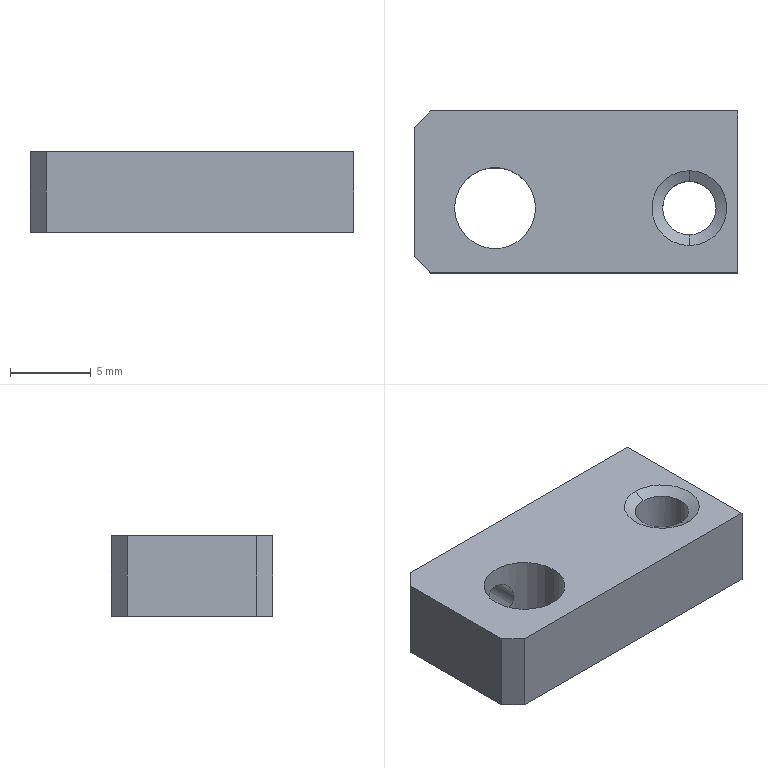Part | NX | 1 solid | 18 faces | box 20 x 10 x 5 mm | volume 834.465 mm3 | plane 8 | cylinder 6 | cone 4 | commonest cylinder face diameters 2.5 x2 3.3 x2 5 x2
STEP:
#1=CARTESIAN_POINT('',(-5.,-3.,0.));
#2=VERTEX_POINT('',#1);
#3=CARTESIAN_POINT('',(-5.,5.,0.));
#4=VERTEX_POINT('',#3);
#5=CARTESIAN_POINT('',(-5.,0.,0.));
#6=DIRECTION('',(0.,1.,0.));
#7=VECTOR('',#6,1000.);
#8=LINE('',#5,#7);
#9=EDGE_CURVE('',#2,#4,#8,.T.);
#10=ORIENTED_EDGE('',*,*,#9,.T.);
#11=CARTESIAN_POINT('',(-4.,6.,0.));
#12=VERTEX_POINT('',#11);
#13=CARTESIAN_POINT('',(-10.,0.,0.));
#14=DIRECTION('',(0.7071,0.7071,0.));
#15=VECTOR('',#14,1000.);
#16=LINE('',#13,#15);
#17=EDGE_CURVE('',#4,#12,#16,.T.);
#18=ORIENTED_EDGE('',*,*,#17,.T.);
#19=CARTESIAN_POINT('',(15.,6.,0.));
#20=VERTEX_POINT('',#19);
#21=CARTESIAN_POINT('',(0.,6.,0.));
#22=DIRECTION('',(-1.,0.,0.));
#23=VECTOR('',#22,1000.);
#24=LINE('',#21,#23);
#25=EDGE_CURVE('',#20,#12,#24,.T.);
#26=ORIENTED_EDGE('',*,*,#25,.F.);
#27=CARTESIAN_POINT('',(15.,-4.,0.));
#28=VERTEX_POINT('',#27);
#29=CARTESIAN_POINT('',(15.,0.,0.));
#30=DIRECTION('',(0.,-1.,0.));
#31=VECTOR('',#30,1000.);
#32=LINE('',#29,#31);
#33=EDGE_CURVE('',#20,#28,#32,.T.);
#34=ORIENTED_EDGE('',*,*,#33,.T.);
#35=CARTESIAN_POINT('',(-4.,-4.,0.));
#36=VERTEX_POINT('',#35);
#37=CARTESIAN_POINT('',(0.,-4.,0.));
#38=DIRECTION('',(-1.,0.,0.));
#39=VECTOR('',#38,1000.);
#40=LINE('',#37,#39);
#41=EDGE_CURVE('',#28,#36,#40,.T.);
#42=ORIENTED_EDGE('',*,*,#41,.T.);
#43=CARTESIAN_POINT('',(-8.,0.,0.));
#44=DIRECTION('',(-0.7071,0.7071,0.));
#45=VECTOR('',#44,1000.);
#46=LINE('',#43,#45);
#47=EDGE_CURVE('',#36,#2,#46,.T.);
#48=ORIENTED_EDGE('',*,*,#47,.T.);
#49=EDGE_LOOP('',(#10,#18,#26,#34,#42,#48));
#50=FACE_BOUND('',#49,.T.);
#51=CARTESIAN_POINT('',(-2.5,0.,0.));
#52=VERTEX_POINT('',#51);
#53=CARTESIAN_POINT('',(2.5,0.,0.));
#54=VERTEX_POINT('',#53);
#55=CARTESIAN_POINT('',(0.,0.,0.));
#56=DIRECTION('',(0.,0.,1.));
#57=DIRECTION('',(1.,0.,0.));
#58=AXIS2_PLACEMENT_3D('',#55,#56,#57);
#59=CIRCLE('',#58,2.5);
#60=EDGE_CURVE('',#52,#54,#59,.T.);
#61=ORIENTED_EDGE('',*,*,#60,.T.);
#62=CARTESIAN_POINT('',(0.,0.,0.));
#63=DIRECTION('',(0.,0.,1.));
#64=DIRECTION('',(1.,0.,0.));
#65=AXIS2_PLACEMENT_3D('',#62,#63,#64);
#66=CIRCLE('',#65,2.5);
#67=EDGE_CURVE('',#54,#52,#66,.T.);
#68=ORIENTED_EDGE('',*,*,#67,.T.);
#69=EDGE_LOOP('',(#61,#68));
#70=FACE_BOUND('',#69,.T.);
#71=CARTESIAN_POINT('',(10.35,0.,0.));
#72=VERTEX_POINT('',#71);
#73=CARTESIAN_POINT('',(13.65,0.,0.));
#74=VERTEX_POINT('',#73);
#75=CARTESIAN_POINT('',(12.,0.,0.));
#76=DIRECTION('',(0.,0.,1.));
#77=DIRECTION('',(-1.,0.,0.));
#78=AXIS2_PLACEMENT_3D('',#75,#76,#77);
#79=CIRCLE('',#78,1.65);
#80=EDGE_CURVE('',#72,#74,#79,.T.);
#81=ORIENTED_EDGE('',*,*,#80,.T.);
#82=CARTESIAN_POINT('',(12.,0.,0.));
#83=DIRECTION('',(0.,0.,1.));
#84=DIRECTION('',(-1.,0.,0.));
#85=AXIS2_PLACEMENT_3D('',#82,#83,#84);
#86=CIRCLE('',#85,1.65);
#87=EDGE_CURVE('',#74,#72,#86,.T.);
#88=ORIENTED_EDGE('',*,*,#87,.T.);
#89=EDGE_LOOP('',(#81,#88));
#90=FACE_BOUND('',#89,.T.);
#91=CARTESIAN_POINT('',(0.,0.,0.));
#92=DIRECTION('',(0.,0.,1.));
#93=DIRECTION('',(1.,0.,0.));
#94=AXIS2_PLACEMENT_3D('',#91,#92,#93);
#95=PLANE('',#94);
#96=ADVANCED_FACE('',(#50,#70,#90),#95,.F.);
#97=ORIENTED_EDGE('',*,*,#9,.F.);
#98=CARTESIAN_POINT('',(-5.,-3.,5.));
#99=VERTEX_POINT('',#98);
#100=CARTESIAN_POINT('',(-5.,-3.,5.));
#101=DIRECTION('',(0.,0.,-1.));
#102=VECTOR('',#101,1000.);
#103=LINE('',#100,#102);
#104=EDGE_CURVE('',#99,#2,#103,.T.);
#105=ORIENTED_EDGE('',*,*,#104,.F.);
#106=CARTESIAN_POINT('',(-5.,5.,5.));
#107=VERTEX_POINT('',#106);
#108=CARTESIAN_POINT('',(-5.,0.,5.));
#109=DIRECTION('',(0.,1.,0.));
#110=VECTOR('',#109,1000.);
#111=LINE('',#108,#110);
#112=EDGE_CURVE('',#99,#107,#111,.T.);
#113=ORIENTED_EDGE('',*,*,#112,.T.);
#114=CARTESIAN_POINT('',(-5.,5.,5.));
#115=DIRECTION('',(0.,0.,-1.));
#116=VECTOR('',#115,1000.);
#117=LINE('',#114,#116);
#118=EDGE_CURVE('',#107,#4,#117,.T.);
#119=ORIENTED_EDGE('',*,*,#118,.T.);
#120=EDGE_LOOP('',(#97,#105,#113,#119));
#121=FACE_BOUND('',#120,.T.);
#122=CARTESIAN_POINT('',(-5.,6.,0.));
#123=DIRECTION('',(-1.,0.,0.));
#124=DIRECTION('',(0.,0.,1.));
#125=AXIS2_PLACEMENT_3D('',#122,#123,#124);
#126=PLANE('',#125);
#127=ADVANCED_FACE('',(#121),#126,.T.);
#128=ORIENTED_EDGE('',*,*,#118,.F.);
#129=CARTESIAN_POINT('',(-4.,6.,5.));
#130=VERTEX_POINT('',#129);
#131=CARTESIAN_POINT('',(-10.,0.,5.));
#132=DIRECTION('',(0.7071,0.7071,0.));
#133=VECTOR('',#132,1000.);
#134=LINE('',#131,#133);
#135=EDGE_CURVE('',#107,#130,#134,.T.);
#136=ORIENTED_EDGE('',*,*,#135,.T.);
#137=CARTESIAN_POINT('',(-4.,6.,0.));
#138=DIRECTION('',(0.,0.,-1.));
#139=VECTOR('',#138,1000.);
#140=LINE('',#137,#139);
#141=EDGE_CURVE('',#130,#12,#140,.T.);
#142=ORIENTED_EDGE('',*,*,#141,.T.);
#143=ORIENTED_EDGE('',*,*,#17,.F.);
#144=EDGE_LOOP('',(#128,#136,#142,#143));
#145=FACE_BOUND('',#144,.T.);
#146=CARTESIAN_POINT('',(-5.,5.,0.));
#147=DIRECTION('',(-0.7071,0.7071,0.));
#148=DIRECTION('',(0.,0.,1.));
#149=AXIS2_PLACEMENT_3D('',#146,#147,#148);
#150=PLANE('',#149);
#151=ADVANCED_FACE('',(#145),#150,.T.);
#152=ORIENTED_EDGE('',*,*,#25,.T.);
#153=ORIENTED_EDGE('',*,*,#141,.F.);
#154=CARTESIAN_POINT('',(15.,6.,5.));
#155=VERTEX_POINT('',#154);
#156=CARTESIAN_POINT('',(0.,6.,5.));
#157=DIRECTION('',(-1.,0.,0.));
#158=VECTOR('',#157,1000.);
#159=LINE('',#156,#158);
#160=EDGE_CURVE('',#155,#130,#159,.T.);
#161=ORIENTED_EDGE('',*,*,#160,.F.);
#162=CARTESIAN_POINT('',(15.,6.,0.));
#163=DIRECTION('',(0.,0.,1.));
#164=VECTOR('',#163,1000.);
#165=LINE('',#162,#164);
#166=EDGE_CURVE('',#20,#155,#165,.T.);
#167=ORIENTED_EDGE('',*,*,#166,.F.);
#168=EDGE_LOOP('',(#152,#153,#161,#167));
#169=FACE_BOUND('',#168,.T.);
#170=CARTESIAN_POINT('',(-1.7,6.,2.5));
#171=VERTEX_POINT('',#170);
#172=CARTESIAN_POINT('',(1.7,6.,2.5));
#173=VERTEX_POINT('',#172);
#174=CARTESIAN_POINT('',(0.,6.,2.5));
#175=DIRECTION('',(0.,1.,0.));
#176=DIRECTION('',(1.,0.,0.));
#177=AXIS2_PLACEMENT_3D('',#174,#175,#176);
#178=CIRCLE('',#177,1.7);
#179=EDGE_CURVE('',#171,#173,#178,.T.);
#180=ORIENTED_EDGE('',*,*,#179,.F.);
#181=CARTESIAN_POINT('',(0.,6.,2.5));
#182=DIRECTION('',(0.,1.,0.));
#183=DIRECTION('',(1.,0.,0.));
#184=AXIS2_PLACEMENT_3D('',#181,#182,#183);
#185=CIRCLE('',#184,1.7);
#186=EDGE_CURVE('',#173,#171,#185,.T.);
#187=ORIENTED_EDGE('',*,*,#186,.F.);
#188=EDGE_LOOP('',(#180,#187));
#189=FACE_BOUND('',#188,.T.);
#190=CARTESIAN_POINT('',(15.,6.,0.));
#191=DIRECTION('',(0.,1.,0.));
#192=DIRECTION('',(1.,0.,0.));
#193=AXIS2_PLACEMENT_3D('',#190,#191,#192);
#194=PLANE('',#193);
#195=ADVANCED_FACE('',(#169,#189),#194,.T.);
#196=ORIENTED_EDGE('',*,*,#33,.F.);
#197=ORIENTED_EDGE('',*,*,#166,.T.);
#198=CARTESIAN_POINT('',(15.,-4.,5.));
#199=VERTEX_POINT('',#198);
#200=CARTESIAN_POINT('',(15.,0.,5.));
#201=DIRECTION('',(0.,-1.,0.));
#202=VECTOR('',#201,1000.);
#203=LINE('',#200,#202);
#204=EDGE_CURVE('',#155,#199,#203,.T.);
#205=ORIENTED_EDGE('',*,*,#204,.T.);
#206=CARTESIAN_POINT('',(15.,-4.,5.));
#207=DIRECTION('',(0.,0.,-1.));
#208=VECTOR('',#207,1000.);
#209=LINE('',#206,#208);
#210=EDGE_CURVE('',#199,#28,#209,.T.);
#211=ORIENTED_EDGE('',*,*,#210,.T.);
#212=EDGE_LOOP('',(#196,#197,#205,#211));
#213=FACE_BOUND('',#212,.T.);
#214=CARTESIAN_POINT('',(15.,-4.,0.));
#215=DIRECTION('',(1.,0.,0.));
#216=DIRECTION('',(0.,1.,0.));
#217=AXIS2_PLACEMENT_3D('',#214,#215,#216);
#218=PLANE('',#217);
#219=ADVANCED_FACE('',(#213),#218,.T.);
#220=ORIENTED_EDGE('',*,*,#41,.F.);
#221=ORIENTED_EDGE('',*,*,#210,.F.);
#222=CARTESIAN_POINT('',(-4.,-4.,5.));
#223=VERTEX_POINT('',#222);
#224=CARTESIAN_POINT('',(0.,-4.,5.));
#225=DIRECTION('',(-1.,0.,0.));
#226=VECTOR('',#225,1000.);
#227=LINE('',#224,#226);
#228=EDGE_CURVE('',#199,#223,#227,.T.);
#229=ORIENTED_EDGE('',*,*,#228,.T.);
#230=CARTESIAN_POINT('',(-4.,-4.,5.));
#231=DIRECTION('',(0.,0.,-1.));
#232=VECTOR('',#231,1000.);
#233=LINE('',#230,#232);
#234=EDGE_CURVE('',#223,#36,#233,.T.);
#235=ORIENTED_EDGE('',*,*,#234,.T.);
#236=EDGE_LOOP('',(#220,#221,#229,#235));
#237=FACE_BOUND('',#236,.T.);
#238=CARTESIAN_POINT('',(-5.,-4.,0.));
#239=DIRECTION('',(0.,-1.,0.));
#240=DIRECTION('',(0.,0.,-1.));
#241=AXIS2_PLACEMENT_3D('',#238,#239,#240);
#242=PLANE('',#241);
#243=ADVANCED_FACE('',(#237),#242,.T.);
#244=ORIENTED_EDGE('',*,*,#234,.F.);
#245=CARTESIAN_POINT('',(-8.,0.,5.));
#246=DIRECTION('',(-0.7071,0.7071,0.));
#247=VECTOR('',#246,1000.);
#248=LINE('',#245,#247);
#249=EDGE_CURVE('',#223,#99,#248,.T.);
#250=ORIENTED_EDGE('',*,*,#249,.T.);
#251=ORIENTED_EDGE('',*,*,#104,.T.);
#252=ORIENTED_EDGE('',*,*,#47,.F.);
#253=EDGE_LOOP('',(#244,#250,#251,#252));
#254=FACE_BOUND('',#253,.T.);
#255=CARTESIAN_POINT('',(-4.,-4.,0.));
#256=DIRECTION('',(-0.7071,-0.7071,0.));
#257=DIRECTION('',(-0.7071,0.7071,0.));
#258=AXIS2_PLACEMENT_3D('',#255,#256,#257);
#259=PLANE('',#258);
#260=ADVANCED_FACE('',(#254),#259,.T.);
#261=ORIENTED_EDGE('',*,*,#112,.F.);
#262=ORIENTED_EDGE('',*,*,#249,.F.);
#263=ORIENTED_EDGE('',*,*,#228,.F.);
#264=ORIENTED_EDGE('',*,*,#204,.F.);
#265=ORIENTED_EDGE('',*,*,#160,.T.);
#266=ORIENTED_EDGE('',*,*,#135,.F.);
#267=EDGE_LOOP('',(#261,#262,#263,#264,#265,#266));
#268=FACE_BOUND('',#267,.T.);
#269=CARTESIAN_POINT('',(-2.5,0.,5.));
#270=VERTEX_POINT('',#269);
#271=CARTESIAN_POINT('',(2.5,0.,5.));
#272=VERTEX_POINT('',#271);
#273=CARTESIAN_POINT('',(0.,0.,5.));
#274=DIRECTION('',(0.,0.,1.));
#275=DIRECTION('',(1.,0.,0.));
#276=AXIS2_PLACEMENT_3D('',#273,#274,#275);
#277=CIRCLE('',#276,2.5);
#278=EDGE_CURVE('',#270,#272,#277,.T.);
#279=ORIENTED_EDGE('',*,*,#278,.F.);
#280=CARTESIAN_POINT('',(0.,0.,5.));
#281=DIRECTION('',(0.,0.,1.));
#282=DIRECTION('',(1.,0.,0.));
#283=AXIS2_PLACEMENT_3D('',#280,#281,#282);
#284=CIRCLE('',#283,2.5);
#285=EDGE_CURVE('',#272,#270,#284,.T.);
#286=ORIENTED_EDGE('',*,*,#285,.F.);
#287=EDGE_LOOP('',(#279,#286));
#288=FACE_BOUND('',#287,.T.);
#289=CARTESIAN_POINT('',(12.,-2.315,5.));
#290=VERTEX_POINT('',#289);
#291=CARTESIAN_POINT('',(12.,2.315,5.));
#292=VERTEX_POINT('',#291);
#293=CARTESIAN_POINT('',(12.,0.,5.));
#294=DIRECTION('',(0.,0.,1.));
#295=DIRECTION('',(0.,1.,0.));
#296=AXIS2_PLACEMENT_3D('',#293,#294,#295);
#297=CIRCLE('',#296,2.315);
#298=EDGE_CURVE('',#290,#292,#297,.T.);
#299=ORIENTED_EDGE('',*,*,#298,.F.);
#300=CARTESIAN_POINT('',(12.,0.,5.));
#301=DIRECTION('',(0.,0.,1.));
#302=DIRECTION('',(0.,1.,0.));
#303=AXIS2_PLACEMENT_3D('',#300,#301,#302);
#304=CIRCLE('',#303,2.315);
#305=EDGE_CURVE('',#292,#290,#304,.T.);
#306=ORIENTED_EDGE('',*,*,#305,.F.);
#307=EDGE_LOOP('',(#299,#306));
#308=FACE_BOUND('',#307,.T.);
#309=CARTESIAN_POINT('',(0.,0.,5.));
#310=DIRECTION('',(0.,0.,1.));
#311=DIRECTION('',(1.,0.,0.));
#312=AXIS2_PLACEMENT_3D('',#309,#310,#311);
#313=PLANE('',#312);
#314=ADVANCED_FACE('',(#268,#288,#308),#313,.T.);
#315=ORIENTED_EDGE('',*,*,#60,.F.);
#316=CARTESIAN_POINT('',(-2.5,0.,0.));
#317=DIRECTION('',(0.,0.,1.));
#318=VECTOR('',#317,1000.);
#319=LINE('',#316,#318);
#320=EDGE_CURVE('',#52,#270,#319,.T.);
#321=ORIENTED_EDGE('',*,*,#320,.T.);
#322=ORIENTED_EDGE('',*,*,#278,.T.);
#323=CARTESIAN_POINT('',(2.5,0.,0.));
#324=DIRECTION('',(0.,0.,1.));
#325=VECTOR('',#324,1000.);
#326=LINE('',#323,#325);
#327=EDGE_CURVE('',#54,#272,#326,.T.);
#328=ORIENTED_EDGE('',*,*,#327,.F.);
#329=EDGE_LOOP('',(#315,#321,#322,#328));
#330=FACE_BOUND('',#329,.T.);
#331=CARTESIAN_POINT('',(0.,0.,0.));
#332=DIRECTION('',(0.,0.,1.));
#333=DIRECTION('',(1.,0.,0.));
#334=AXIS2_PLACEMENT_3D('',#331,#332,#333);
#335=CYLINDRICAL_SURFACE('',#334,2.5);
#336=ADVANCED_FACE('',(#330),#335,.F.);
#337=ORIENTED_EDGE('',*,*,#298,.T.);
#338=CARTESIAN_POINT('',(12.,1.65,4.616));
#339=VERTEX_POINT('',#338);
#340=CARTESIAN_POINT('',(12.,2.315,5.));
#341=DIRECTION('',(0.,0.866,0.5));
#342=VECTOR('',#341,1000.);
#343=LINE('',#340,#342);
#344=EDGE_CURVE('',#339,#292,#343,.T.);
#345=ORIENTED_EDGE('',*,*,#344,.F.);
#346=CARTESIAN_POINT('',(13.65,0.,4.616));
#347=VERTEX_POINT('',#346);
#348=CARTESIAN_POINT('',(12.,0.,4.616));
#349=DIRECTION('',(0.,0.,1.));
#350=DIRECTION('',(0.,1.,0.));
#351=AXIS2_PLACEMENT_3D('',#348,#349,#350);
#352=CIRCLE('',#351,1.65);
#353=EDGE_CURVE('',#347,#339,#352,.T.);
#354=ORIENTED_EDGE('',*,*,#353,.F.);
#355=CARTESIAN_POINT('',(12.,-1.65,4.616));
#356=VERTEX_POINT('',#355);
#357=CARTESIAN_POINT('',(12.,0.,4.616));
#358=DIRECTION('',(0.,0.,1.));
#359=DIRECTION('',(0.,1.,0.));
#360=AXIS2_PLACEMENT_3D('',#357,#358,#359);
#361=CIRCLE('',#360,1.65);
#362=EDGE_CURVE('',#356,#347,#361,.T.);
#363=ORIENTED_EDGE('',*,*,#362,.F.);
#364=CARTESIAN_POINT('',(12.,-2.315,5.));
#365=DIRECTION('',(0.,-0.866,0.5));
#366=VECTOR('',#365,1000.);
#367=LINE('',#364,#366);
#368=EDGE_CURVE('',#356,#290,#367,.T.);
#369=ORIENTED_EDGE('',*,*,#368,.T.);
#370=EDGE_LOOP('',(#337,#345,#354,#363,#369));
#371=FACE_BOUND('',#370,.T.);
#372=CARTESIAN_POINT('',(12.,0.,5.));
#373=DIRECTION('',(0.,0.,1.));
#374=DIRECTION('',(0.,1.,0.));
#375=AXIS2_PLACEMENT_3D('',#372,#373,#374);
#376=CONICAL_SURFACE('',#375,2.315,1.047);
#377=ADVANCED_FACE('',(#371),#376,.F.);
#378=ORIENTED_EDGE('',*,*,#80,.F.);
#379=CARTESIAN_POINT('',(10.35,0.,4.616));
#380=VERTEX_POINT('',#379);
#381=CARTESIAN_POINT('',(10.35,0.,2.5));
#382=DIRECTION('',(0.,0.,1.));
#383=VECTOR('',#382,1000.);
#384=LINE('',#381,#383);
#385=EDGE_CURVE('',#72,#380,#384,.T.);
#386=ORIENTED_EDGE('',*,*,#385,.T.);
#387=CARTESIAN_POINT('',(12.,0.,4.616));
#388=DIRECTION('',(0.,0.,1.));
#389=DIRECTION('',(0.,1.,0.));
#390=AXIS2_PLACEMENT_3D('',#387,#388,#389);
#391=CIRCLE('',#390,1.65);
#392=EDGE_CURVE('',#380,#356,#391,.T.);
#393=ORIENTED_EDGE('',*,*,#392,.T.);
#394=ORIENTED_EDGE('',*,*,#362,.T.);
#395=CARTESIAN_POINT('',(13.65,0.,2.5));
#396=DIRECTION('',(0.,0.,1.));
#397=VECTOR('',#396,1000.);
#398=LINE('',#395,#397);
#399=EDGE_CURVE('',#74,#347,#398,.T.);
#400=ORIENTED_EDGE('',*,*,#399,.F.);
#401=EDGE_LOOP('',(#378,#386,#393,#394,#400));
#402=FACE_BOUND('',#401,.T.);
#403=CARTESIAN_POINT('',(12.,0.,2.5));
#404=DIRECTION('',(0.,0.,1.));
#405=DIRECTION('',(-1.,0.,0.));
#406=AXIS2_PLACEMENT_3D('',#403,#404,#405);
#407=CYLINDRICAL_SURFACE('',#406,1.65);
#408=ADVANCED_FACE('',(#402),#407,.F.);
#409=CARTESIAN_POINT('',(1.25,2.165,2.5));
#410=VERTEX_POINT('',#409);
#411=CARTESIAN_POINT('',(-1.25,2.165,2.5));
#412=VERTEX_POINT('',#411);
#413=CARTESIAN_POINT('',(-1.25,2.165,2.5));
#414=CARTESIAN_POINT('',(-1.25,2.165,2.346));
#415=CARTESIAN_POINT('',(-1.174,2.207,2.041));
#416=CARTESIAN_POINT('',(-1.086,2.254,1.868));
#417=CARTESIAN_POINT('',(-0.8902,2.341,1.6));
#418=CARTESIAN_POINT('',(-0.6604,2.413,1.432));
#419=CARTESIAN_POINT('',(-0.4382,2.467,1.316));
#420=CARTESIAN_POINT('',(0.0000852,2.522,1.206));
#421=CARTESIAN_POINT('',(0.438,2.467,1.316));
#422=CARTESIAN_POINT('',(0.6602,2.413,1.432));
#423=CARTESIAN_POINT('',(0.8905,2.34,1.601));
#424=CARTESIAN_POINT('',(1.086,2.254,1.868));
#425=CARTESIAN_POINT('',(1.174,2.207,2.041));
#426=CARTESIAN_POINT('',(1.25,2.165,2.346));
#427=CARTESIAN_POINT('',(1.25,2.165,2.5));
#428=B_SPLINE_CURVE_WITH_KNOTS('',3,(#413,#414,#415,#416,#417,#418,#419,#420,#421,#422,#423,#424,#425,#426,#427),.UNSPECIFIED.,.F.,.F.,(4,1,1,1,1,1,1,1,1,1,1,1,4),(0.,0.125,0.1875,0.25,0.3125,0.375,0.5,0.625,0.6875,0.75,0.8125,0.875,1.),.UNSPECIFIED.);
#429=EDGE_CURVE('',#410,#412,#428,.F.);
#430=ORIENTED_EDGE('',*,*,#429,.F.);
#431=CARTESIAN_POINT('',(1.25,5.74,2.5));
#432=VERTEX_POINT('',#431);
#433=CARTESIAN_POINT('',(1.25,4.083,2.5));
#434=DIRECTION('',(0.,1.,0.));
#435=VECTOR('',#434,1000.);
#436=LINE('',#433,#435);
#437=EDGE_CURVE('',#410,#432,#436,.T.);
#438=ORIENTED_EDGE('',*,*,#437,.T.);
#439=CARTESIAN_POINT('',(-1.25,5.74,2.5));
#440=VERTEX_POINT('',#439);
#441=CARTESIAN_POINT('',(0.,5.74,2.5));
#442=DIRECTION('',(0.,1.,0.));
#443=DIRECTION('',(1.,0.,0.));
#444=AXIS2_PLACEMENT_3D('',#441,#442,#443);
#445=CIRCLE('',#444,1.25);
#446=EDGE_CURVE('',#432,#440,#445,.T.);
#447=ORIENTED_EDGE('',*,*,#446,.T.);
#448=CARTESIAN_POINT('',(-1.25,4.083,2.5));
#449=DIRECTION('',(0.,1.,0.));
#450=VECTOR('',#449,1000.);
#451=LINE('',#448,#450);
#452=EDGE_CURVE('',#412,#440,#451,.T.);
#453=ORIENTED_EDGE('',*,*,#452,.F.);
#454=EDGE_LOOP('',(#430,#438,#447,#453));
#455=FACE_BOUND('',#454,.T.);
#456=CARTESIAN_POINT('',(0.,4.083,2.5));
#457=DIRECTION('',(0.,1.,0.));
#458=DIRECTION('',(1.,0.,0.));
#459=AXIS2_PLACEMENT_3D('',#456,#457,#458);
#460=CYLINDRICAL_SURFACE('',#459,1.25);
#461=ADVANCED_FACE('',(#455),#460,.F.);
#462=ORIENTED_EDGE('',*,*,#179,.T.);
#463=CARTESIAN_POINT('',(1.25,5.74,2.5));
#464=DIRECTION('',(0.866,0.5,0.));
#465=VECTOR('',#464,1000.);
#466=LINE('',#463,#465);
#467=EDGE_CURVE('',#432,#173,#466,.T.);
#468=ORIENTED_EDGE('',*,*,#467,.F.);
#469=CARTESIAN_POINT('',(0.,5.74,2.5));
#470=DIRECTION('',(0.,1.,0.));
#471=DIRECTION('',(1.,0.,0.));
#472=AXIS2_PLACEMENT_3D('',#469,#470,#471);
#473=CIRCLE('',#472,1.25);
#474=EDGE_CURVE('',#440,#432,#473,.T.);
#475=ORIENTED_EDGE('',*,*,#474,.F.);
#476=CARTESIAN_POINT('',(-1.25,5.74,2.5));
#477=DIRECTION('',(-0.866,0.5,0.));
#478=VECTOR('',#477,1000.);
#479=LINE('',#476,#478);
#480=EDGE_CURVE('',#440,#171,#479,.T.);
#481=ORIENTED_EDGE('',*,*,#480,.T.);
#482=EDGE_LOOP('',(#462,#468,#475,#481));
#483=FACE_BOUND('',#482,.T.);
#484=CARTESIAN_POINT('',(0.,5.74,2.5));
#485=DIRECTION('',(0.,1.,0.));
#486=DIRECTION('',(1.,0.,0.));
#487=AXIS2_PLACEMENT_3D('',#484,#485,#486);
#488=CONICAL_SURFACE('',#487,1.25,1.047);
#489=ADVANCED_FACE('',(#483),#488,.F.);
#490=ORIENTED_EDGE('',*,*,#437,.F.);
#491=CARTESIAN_POINT('',(1.25,2.165,2.5));
#492=CARTESIAN_POINT('',(1.25,2.165,2.654));
#493=CARTESIAN_POINT('',(1.174,2.207,2.959));
#494=CARTESIAN_POINT('',(1.086,2.254,3.132));
#495=CARTESIAN_POINT('',(0.8903,2.34,3.4));
#496=CARTESIAN_POINT('',(0.6605,2.413,3.568));
#497=CARTESIAN_POINT('',(0.4382,2.467,3.684));
#498=CARTESIAN_POINT('',(-0.000141,2.522,3.794));
#499=CARTESIAN_POINT('',(-0.4378,2.467,3.684));
#500=CARTESIAN_POINT('',(-0.6602,2.413,3.568));
#501=CARTESIAN_POINT('',(-0.8904,2.34,3.399));
#502=CARTESIAN_POINT('',(-1.086,2.254,3.132));
#503=CARTESIAN_POINT('',(-1.174,2.207,2.959));
#504=CARTESIAN_POINT('',(-1.25,2.165,2.654));
#505=CARTESIAN_POINT('',(-1.25,2.165,2.5));
#506=B_SPLINE_CURVE_WITH_KNOTS('',3,(#491,#492,#493,#494,#495,#496,#497,#498,#499,#500,#501,#502,#503,#504,#505),.UNSPECIFIED.,.F.,.F.,(4,1,1,1,1,1,1,1,1,1,1,1,4),(0.,0.125,0.1875,0.25,0.3125,0.375,0.5,0.625,0.6875,0.75,0.8125,0.875,1.),.UNSPECIFIED.);
#507=EDGE_CURVE('',#412,#410,#506,.F.);
#508=ORIENTED_EDGE('',*,*,#507,.F.);
#509=ORIENTED_EDGE('',*,*,#452,.T.);
#510=ORIENTED_EDGE('',*,*,#474,.T.);
#511=EDGE_LOOP('',(#490,#508,#509,#510));
#512=FACE_BOUND('',#511,.T.);
#513=CARTESIAN_POINT('',(0.,4.083,2.5));
#514=DIRECTION('',(0.,1.,0.));
#515=DIRECTION('',(1.,0.,0.));
#516=AXIS2_PLACEMENT_3D('',#513,#514,#515);
#517=CYLINDRICAL_SURFACE('',#516,1.25);
#518=ADVANCED_FACE('',(#512),#517,.F.);
#519=ORIENTED_EDGE('',*,*,#399,.T.);
#520=ORIENTED_EDGE('',*,*,#353,.T.);
#521=CARTESIAN_POINT('',(12.,0.,4.616));
#522=DIRECTION('',(0.,0.,1.));
#523=DIRECTION('',(0.,1.,0.));
#524=AXIS2_PLACEMENT_3D('',#521,#522,#523);
#525=CIRCLE('',#524,1.65);
#526=EDGE_CURVE('',#339,#380,#525,.T.);
#527=ORIENTED_EDGE('',*,*,#526,.T.);
#528=ORIENTED_EDGE('',*,*,#385,.F.);
#529=ORIENTED_EDGE('',*,*,#87,.F.);
#530=EDGE_LOOP('',(#519,#520,#527,#528,#529));
#531=FACE_BOUND('',#530,.T.);
#532=CARTESIAN_POINT('',(12.,0.,2.5));
#533=DIRECTION('',(0.,0.,1.));
#534=DIRECTION('',(-1.,0.,0.));
#535=AXIS2_PLACEMENT_3D('',#532,#533,#534);
#536=CYLINDRICAL_SURFACE('',#535,1.65);
#537=ADVANCED_FACE('',(#531),#536,.F.);
#538=ORIENTED_EDGE('',*,*,#446,.F.);
#539=ORIENTED_EDGE('',*,*,#467,.T.);
#540=ORIENTED_EDGE('',*,*,#186,.T.);
#541=ORIENTED_EDGE('',*,*,#480,.F.);
#542=EDGE_LOOP('',(#538,#539,#540,#541));
#543=FACE_BOUND('',#542,.T.);
#544=CARTESIAN_POINT('',(0.,5.74,2.5));
#545=DIRECTION('',(0.,1.,0.));
#546=DIRECTION('',(1.,0.,0.));
#547=AXIS2_PLACEMENT_3D('',#544,#545,#546);
#548=CONICAL_SURFACE('',#547,1.25,1.047);
#549=ADVANCED_FACE('',(#543),#548,.F.);
#550=ORIENTED_EDGE('',*,*,#392,.F.);
#551=ORIENTED_EDGE('',*,*,#526,.F.);
#552=ORIENTED_EDGE('',*,*,#344,.T.);
#553=ORIENTED_EDGE('',*,*,#305,.T.);
#554=ORIENTED_EDGE('',*,*,#368,.F.);
#555=EDGE_LOOP('',(#550,#551,#552,#553,#554));
#556=FACE_BOUND('',#555,.T.);
#557=CARTESIAN_POINT('',(12.,0.,5.));
#558=DIRECTION('',(0.,0.,1.));
#559=DIRECTION('',(0.,1.,0.));
#560=AXIS2_PLACEMENT_3D('',#557,#558,#559);
#561=CONICAL_SURFACE('',#560,2.315,1.047);
#562=ADVANCED_FACE('',(#556),#561,.F.);
#563=ORIENTED_EDGE('',*,*,#327,.T.);
#564=ORIENTED_EDGE('',*,*,#285,.T.);
#565=ORIENTED_EDGE('',*,*,#320,.F.);
#566=ORIENTED_EDGE('',*,*,#67,.F.);
#567=EDGE_LOOP('',(#563,#564,#565,#566));
#568=FACE_BOUND('',#567,.T.);
#569=ORIENTED_EDGE('',*,*,#429,.T.);
#570=ORIENTED_EDGE('',*,*,#507,.T.);
#571=EDGE_LOOP('',(#569,#570));
#572=FACE_BOUND('',#571,.T.);
#573=CARTESIAN_POINT('',(0.,0.,0.));
#574=DIRECTION('',(0.,0.,1.));
#575=DIRECTION('',(1.,0.,0.));
#576=AXIS2_PLACEMENT_3D('',#573,#574,#575);
#577=CYLINDRICAL_SURFACE('',#576,2.5);
#578=ADVANCED_FACE('',(#568,#572),#577,.F.);
#579=CLOSED_SHELL('',(#96,#127,#151,#195,#219,#243,#260,#314,#336,#377,#408,#461,#489,#518,#537,#549,#562,#578));
#580=MANIFOLD_SOLID_BREP('',#579);
#581=(LENGTH_UNIT()NAMED_UNIT(*)SI_UNIT(.MILLI.,.METRE.));
#582=UNCERTAINTY_MEASURE_WITH_UNIT(LENGTH_MEASURE(0.0508),#581,'','');
#583=(NAMED_UNIT(*)PLANE_ANGLE_UNIT()SI_UNIT($,.RADIAN.));
#584=(NAMED_UNIT(*)SI_UNIT($,.STERADIAN.)SOLID_ANGLE_UNIT());
#585=(GEOMETRIC_REPRESENTATION_CONTEXT(3)GLOBAL_UNCERTAINTY_ASSIGNED_CONTEXT((#582))GLOBAL_UNIT_ASSIGNED_CONTEXT((#581,#583,#584))REPRESENTATION_CONTEXT('',''));
#586=ADVANCED_BREP_SHAPE_REPRESENTATION('',(#580),#585);